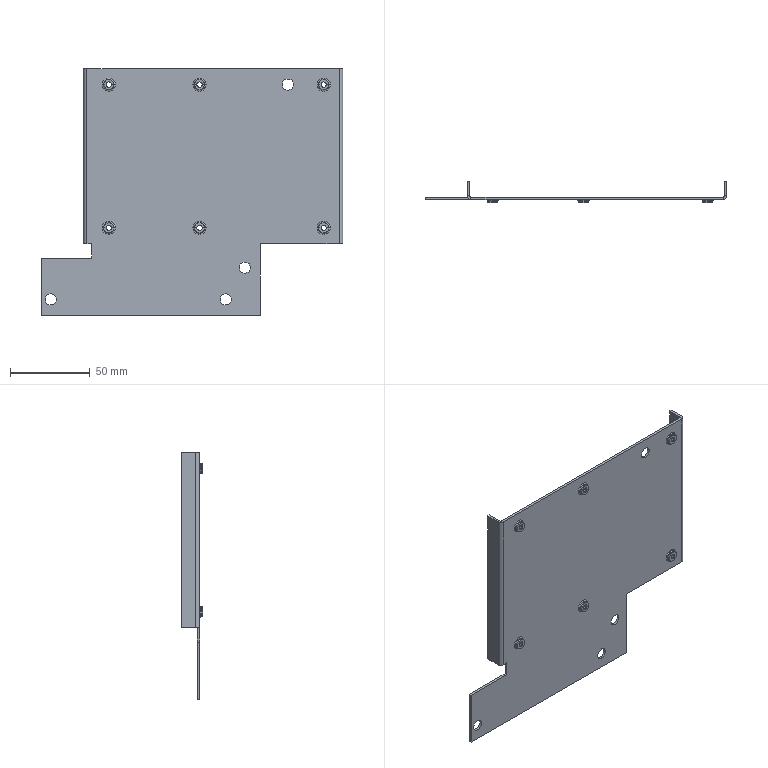Part | STEP file | 68374120 | 1 solid | 120 faces | box 189.45 x 13.5 x 155 mm | volume 38724 mm3 | torus 48 | plane 36 | cylinder 36 | commonest cylinder face diameters 3.3 x12 6.3 x12 7 x8 1.6 x2 4.6 x2